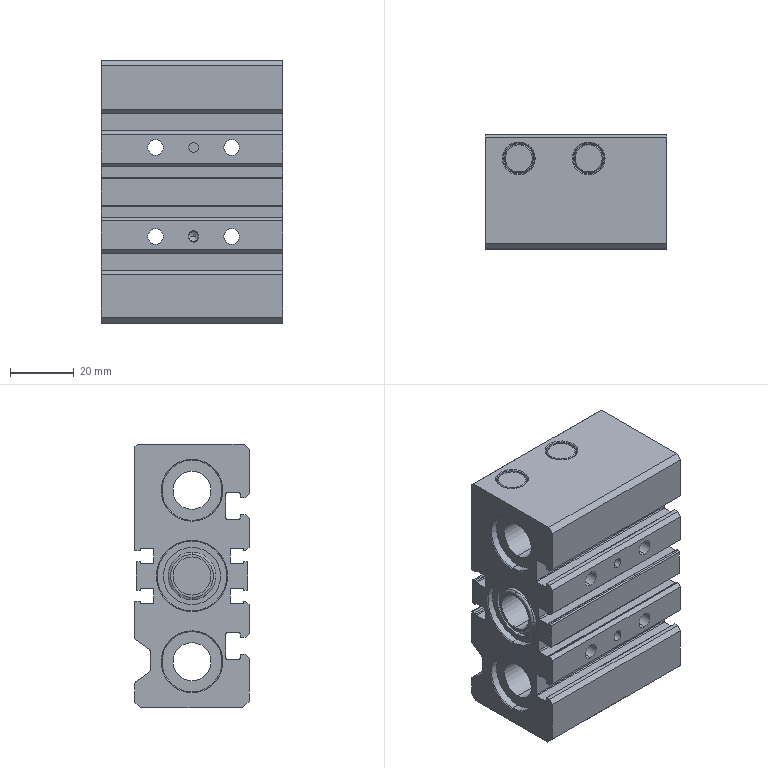Part | STEP file | 11-_TC-M-20x2020_b11 | 1 solid | 287 faces | box 57 x 36 x 83 mm | volume 110074 mm3 | cylinder 130 | plane 95 | cone 60 | spline 2 | commonest cylinder face diameters 0.8 x20 3 x14 0.4 x12 0.6 x10 4.134 x8 4.917 x8